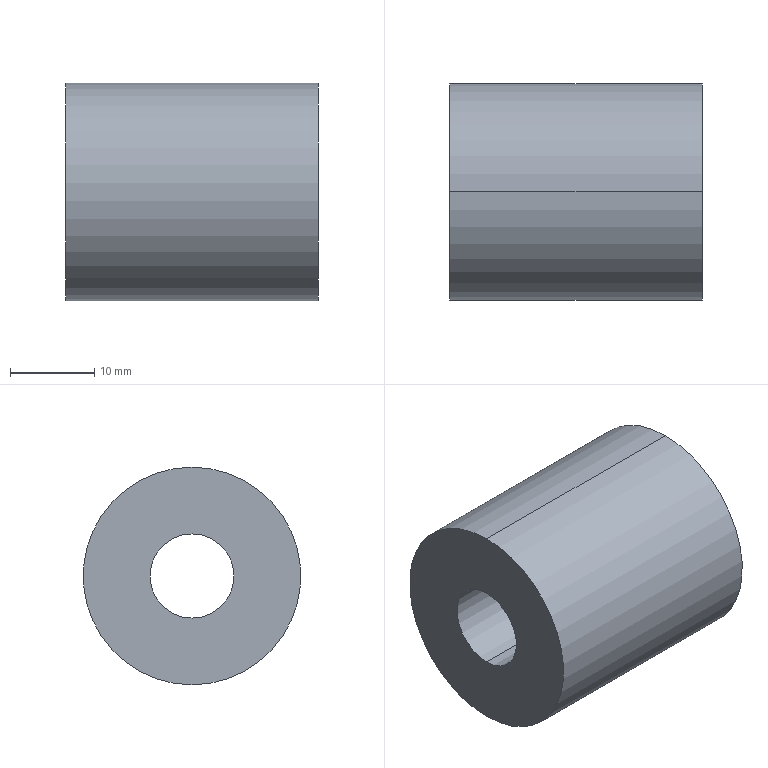Part | SolidWorks | features BaseBody 1 | 1 solid | 6 faces | box 30 x 25.832 x 25.832 mm | volume 13367 mm3 | cylinder 4 | plane 2 | commonest cylinder face diameters 10 x2 25.832 x2
STEP:
#1=CARTESIAN_POINT('',(-104.,23.,44.916));
#2=VERTEX_POINT('',#1);
#3=CARTESIAN_POINT('',(-104.,23.,19.084));
#4=VERTEX_POINT('',#3);
#5=CARTESIAN_POINT('',(-104.,23.,32.));
#6=DIRECTION('',(-1.,0.,0.));
#7=DIRECTION('',(0.,0.,1.));
#8=AXIS2_PLACEMENT_3D('',#5,#6,#7);
#9=CIRCLE('',#8,12.916);
#10=EDGE_CURVE('',#2,#4,#9,.T.);
#11=ORIENTED_EDGE('',*,*,#10,.T.);
#12=CARTESIAN_POINT('',(-134.,23.,19.084));
#13=VERTEX_POINT('',#12);
#14=CARTESIAN_POINT('',(-104.,23.,19.084));
#15=DIRECTION('',(-1.,0.,0.));
#16=VECTOR('',#15,1000.);
#17=LINE('',#14,#16);
#18=EDGE_CURVE('',#4,#13,#17,.T.);
#19=ORIENTED_EDGE('',*,*,#18,.T.);
#20=CARTESIAN_POINT('',(-134.,23.,44.916));
#21=VERTEX_POINT('',#20);
#22=CARTESIAN_POINT('',(-134.,23.,32.));
#23=DIRECTION('',(1.,0.,0.));
#24=DIRECTION('',(0.,0.,1.));
#25=AXIS2_PLACEMENT_3D('',#22,#23,#24);
#26=CIRCLE('',#25,12.916);
#27=EDGE_CURVE('',#13,#21,#26,.T.);
#28=ORIENTED_EDGE('',*,*,#27,.T.);
#29=CARTESIAN_POINT('',(-104.,23.,44.916));
#30=DIRECTION('',(-1.,0.,0.));
#31=VECTOR('',#30,1000.);
#32=LINE('',#29,#31);
#33=EDGE_CURVE('',#2,#21,#32,.T.);
#34=ORIENTED_EDGE('',*,*,#33,.F.);
#35=EDGE_LOOP('',(#11,#19,#28,#34));
#36=FACE_OUTER_BOUND('',#35,.T.);
#37=CARTESIAN_POINT('',(-104.,23.,32.));
#38=DIRECTION('',(-1.,0.,0.));
#39=DIRECTION('',(0.,0.,1.));
#40=AXIS2_PLACEMENT_3D('',#37,#38,#39);
#41=CYLINDRICAL_SURFACE('',#40,12.916);
#42=ADVANCED_FACE('',(#36),#41,.T.);
#43=CARTESIAN_POINT('',(-104.,23.,27.));
#44=VERTEX_POINT('',#43);
#45=CARTESIAN_POINT('',(-104.,23.,37.));
#46=VERTEX_POINT('',#45);
#47=CARTESIAN_POINT('',(-104.,23.,32.));
#48=DIRECTION('',(-1.,0.,0.));
#49=DIRECTION('',(0.,0.,1.));
#50=AXIS2_PLACEMENT_3D('',#47,#48,#49);
#51=CIRCLE('',#50,5.);
#52=EDGE_CURVE('',#44,#46,#51,.T.);
#53=ORIENTED_EDGE('',*,*,#52,.F.);
#54=CARTESIAN_POINT('',(-134.,23.,27.));
#55=VERTEX_POINT('',#54);
#56=CARTESIAN_POINT('',(-104.,23.,27.));
#57=DIRECTION('',(-1.,0.,0.));
#58=VECTOR('',#57,1000.);
#59=LINE('',#56,#58);
#60=EDGE_CURVE('',#44,#55,#59,.T.);
#61=ORIENTED_EDGE('',*,*,#60,.T.);
#62=CARTESIAN_POINT('',(-134.,23.,37.));
#63=VERTEX_POINT('',#62);
#64=CARTESIAN_POINT('',(-134.,23.,32.));
#65=DIRECTION('',(-1.,0.,0.));
#66=DIRECTION('',(0.,0.,1.));
#67=AXIS2_PLACEMENT_3D('',#64,#65,#66);
#68=CIRCLE('',#67,5.);
#69=EDGE_CURVE('',#55,#63,#68,.T.);
#70=ORIENTED_EDGE('',*,*,#69,.T.);
#71=CARTESIAN_POINT('',(-104.,23.,37.));
#72=DIRECTION('',(-1.,0.,0.));
#73=VECTOR('',#72,1000.);
#74=LINE('',#71,#73);
#75=EDGE_CURVE('',#46,#63,#74,.T.);
#76=ORIENTED_EDGE('',*,*,#75,.F.);
#77=EDGE_LOOP('',(#53,#61,#70,#76));
#78=FACE_OUTER_BOUND('',#77,.T.);
#79=CARTESIAN_POINT('',(-104.,23.,32.));
#80=DIRECTION('',(-1.,0.,0.));
#81=DIRECTION('',(0.,0.,1.));
#82=AXIS2_PLACEMENT_3D('',#79,#80,#81);
#83=CYLINDRICAL_SURFACE('',#82,5.);
#84=ADVANCED_FACE('',(#78),#83,.F.);
#85=ORIENTED_EDGE('',*,*,#18,.F.);
#86=CARTESIAN_POINT('',(-104.,23.,32.));
#87=DIRECTION('',(-1.,0.,0.));
#88=DIRECTION('',(0.,0.,1.));
#89=AXIS2_PLACEMENT_3D('',#86,#87,#88);
#90=CIRCLE('',#89,12.916);
#91=EDGE_CURVE('',#4,#2,#90,.T.);
#92=ORIENTED_EDGE('',*,*,#91,.T.);
#93=ORIENTED_EDGE('',*,*,#33,.T.);
#94=CARTESIAN_POINT('',(-134.,23.,32.));
#95=DIRECTION('',(1.,0.,0.));
#96=DIRECTION('',(0.,0.,1.));
#97=AXIS2_PLACEMENT_3D('',#94,#95,#96);
#98=CIRCLE('',#97,12.916);
#99=EDGE_CURVE('',#21,#13,#98,.T.);
#100=ORIENTED_EDGE('',*,*,#99,.T.);
#101=EDGE_LOOP('',(#85,#92,#93,#100));
#102=FACE_OUTER_BOUND('',#101,.T.);
#103=CARTESIAN_POINT('',(-104.,23.,32.));
#104=DIRECTION('',(-1.,0.,0.));
#105=DIRECTION('',(0.,0.,1.));
#106=AXIS2_PLACEMENT_3D('',#103,#104,#105);
#107=CYLINDRICAL_SURFACE('',#106,12.916);
#108=ADVANCED_FACE('',(#102),#107,.T.);
#109=CARTESIAN_POINT('',(-104.,23.,32.));
#110=DIRECTION('',(-1.,0.,0.));
#111=DIRECTION('',(0.,0.,1.));
#112=AXIS2_PLACEMENT_3D('',#109,#110,#111);
#113=CIRCLE('',#112,5.);
#114=EDGE_CURVE('',#46,#44,#113,.T.);
#115=ORIENTED_EDGE('',*,*,#114,.T.);
#116=ORIENTED_EDGE('',*,*,#52,.T.);
#117=EDGE_LOOP('',(#115,#116));
#118=FACE_BOUND('',#117,.T.);
#119=ORIENTED_EDGE('',*,*,#10,.F.);
#120=ORIENTED_EDGE('',*,*,#91,.F.);
#121=EDGE_LOOP('',(#119,#120));
#122=FACE_OUTER_BOUND('',#121,.T.);
#123=CARTESIAN_POINT('',(-104.,23.,32.));
#124=DIRECTION('',(1.,0.,0.));
#125=DIRECTION('',(0.,0.,-1.));
#126=AXIS2_PLACEMENT_3D('',#123,#124,#125);
#127=PLANE('',#126);
#128=ADVANCED_FACE('',(#118,#122),#127,.T.);
#129=CARTESIAN_POINT('',(-134.,23.,32.));
#130=DIRECTION('',(-1.,0.,0.));
#131=DIRECTION('',(0.,0.,1.));
#132=AXIS2_PLACEMENT_3D('',#129,#130,#131);
#133=CIRCLE('',#132,5.);
#134=EDGE_CURVE('',#63,#55,#133,.T.);
#135=ORIENTED_EDGE('',*,*,#134,.F.);
#136=ORIENTED_EDGE('',*,*,#69,.F.);
#137=EDGE_LOOP('',(#135,#136));
#138=FACE_BOUND('',#137,.T.);
#139=ORIENTED_EDGE('',*,*,#99,.F.);
#140=ORIENTED_EDGE('',*,*,#27,.F.);
#141=EDGE_LOOP('',(#139,#140));
#142=FACE_OUTER_BOUND('',#141,.T.);
#143=CARTESIAN_POINT('',(-134.,23.,32.));
#144=DIRECTION('',(1.,0.,0.));
#145=DIRECTION('',(0.,0.,-1.));
#146=AXIS2_PLACEMENT_3D('',#143,#144,#145);
#147=PLANE('',#146);
#148=ADVANCED_FACE('',(#138,#142),#147,.F.);
#149=ORIENTED_EDGE('',*,*,#60,.F.);
#150=ORIENTED_EDGE('',*,*,#114,.F.);
#151=ORIENTED_EDGE('',*,*,#75,.T.);
#152=ORIENTED_EDGE('',*,*,#134,.T.);
#153=EDGE_LOOP('',(#149,#150,#151,#152));
#154=FACE_OUTER_BOUND('',#153,.T.);
#155=CARTESIAN_POINT('',(-104.,23.,32.));
#156=DIRECTION('',(-1.,0.,0.));
#157=DIRECTION('',(0.,0.,1.));
#158=AXIS2_PLACEMENT_3D('',#155,#156,#157);
#159=CYLINDRICAL_SURFACE('',#158,5.);
#160=ADVANCED_FACE('',(#154),#159,.F.);
#161=CLOSED_SHELL('',(#42,#84,#108,#128,#148,#160));
#162=MANIFOLD_SOLID_BREP('',#161);
#163=CARTESIAN_POINT('',(0.,0.,0.));
#164=DIRECTION('',(0.,0.,1.));
#165=DIRECTION('',(1.,0.,0.));
#166=AXIS2_PLACEMENT_3D('',#163,#164,#165);
#167=(LENGTH_UNIT()NAMED_UNIT(*)SI_UNIT(.MILLI.,.METRE.));
#168=UNCERTAINTY_MEASURE_WITH_UNIT(LENGTH_MEASURE(0.00001),#167,'','');
#169=(NAMED_UNIT(*)PLANE_ANGLE_UNIT()SI_UNIT($,.RADIAN.));
#170=(NAMED_UNIT(*)SI_UNIT($,.STERADIAN.)SOLID_ANGLE_UNIT());
#171=(GEOMETRIC_REPRESENTATION_CONTEXT(3)GLOBAL_UNCERTAINTY_ASSIGNED_CONTEXT((#168))GLOBAL_UNIT_ASSIGNED_CONTEXT((#167,#169,#170))REPRESENTATION_CONTEXT('',''));
#172=ADVANCED_BREP_SHAPE_REPRESENTATION('',(#162,#166),#171);